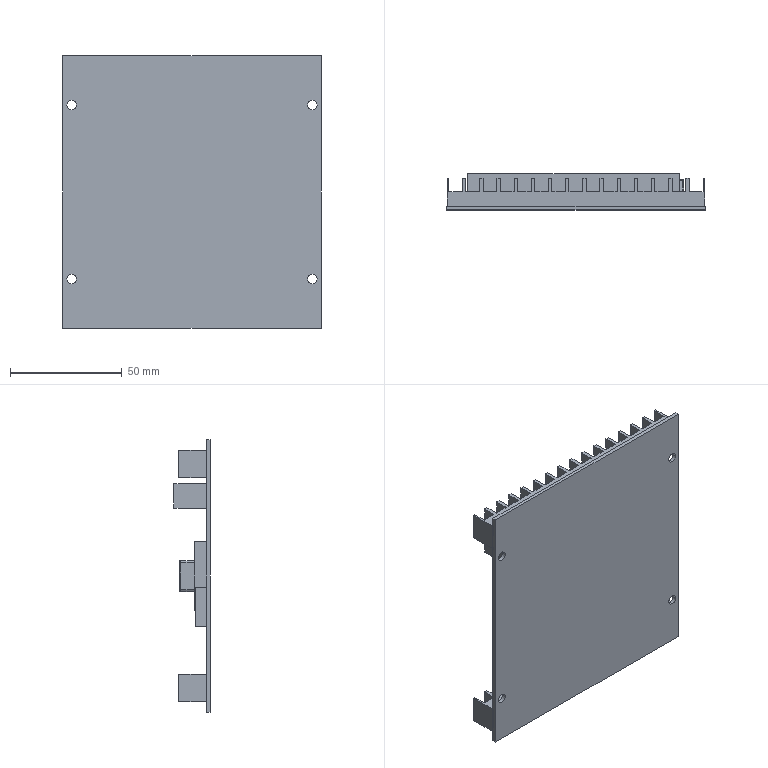Part | STEP file | Large sheet machine | 1 solid | 182 faces | box 116 x 16.2 x 122 mm | volume 66720 mm3 | plane 158 | cylinder 20 | spline 2 | torus 2 | commonest cylinder face diameters 4.2 x8 1 x4 2 x4 3 x4